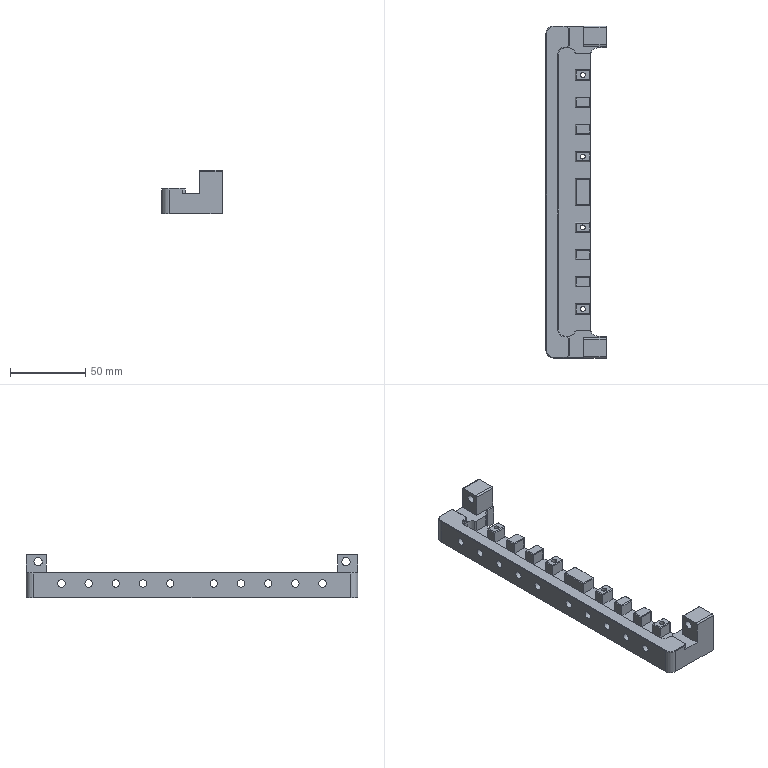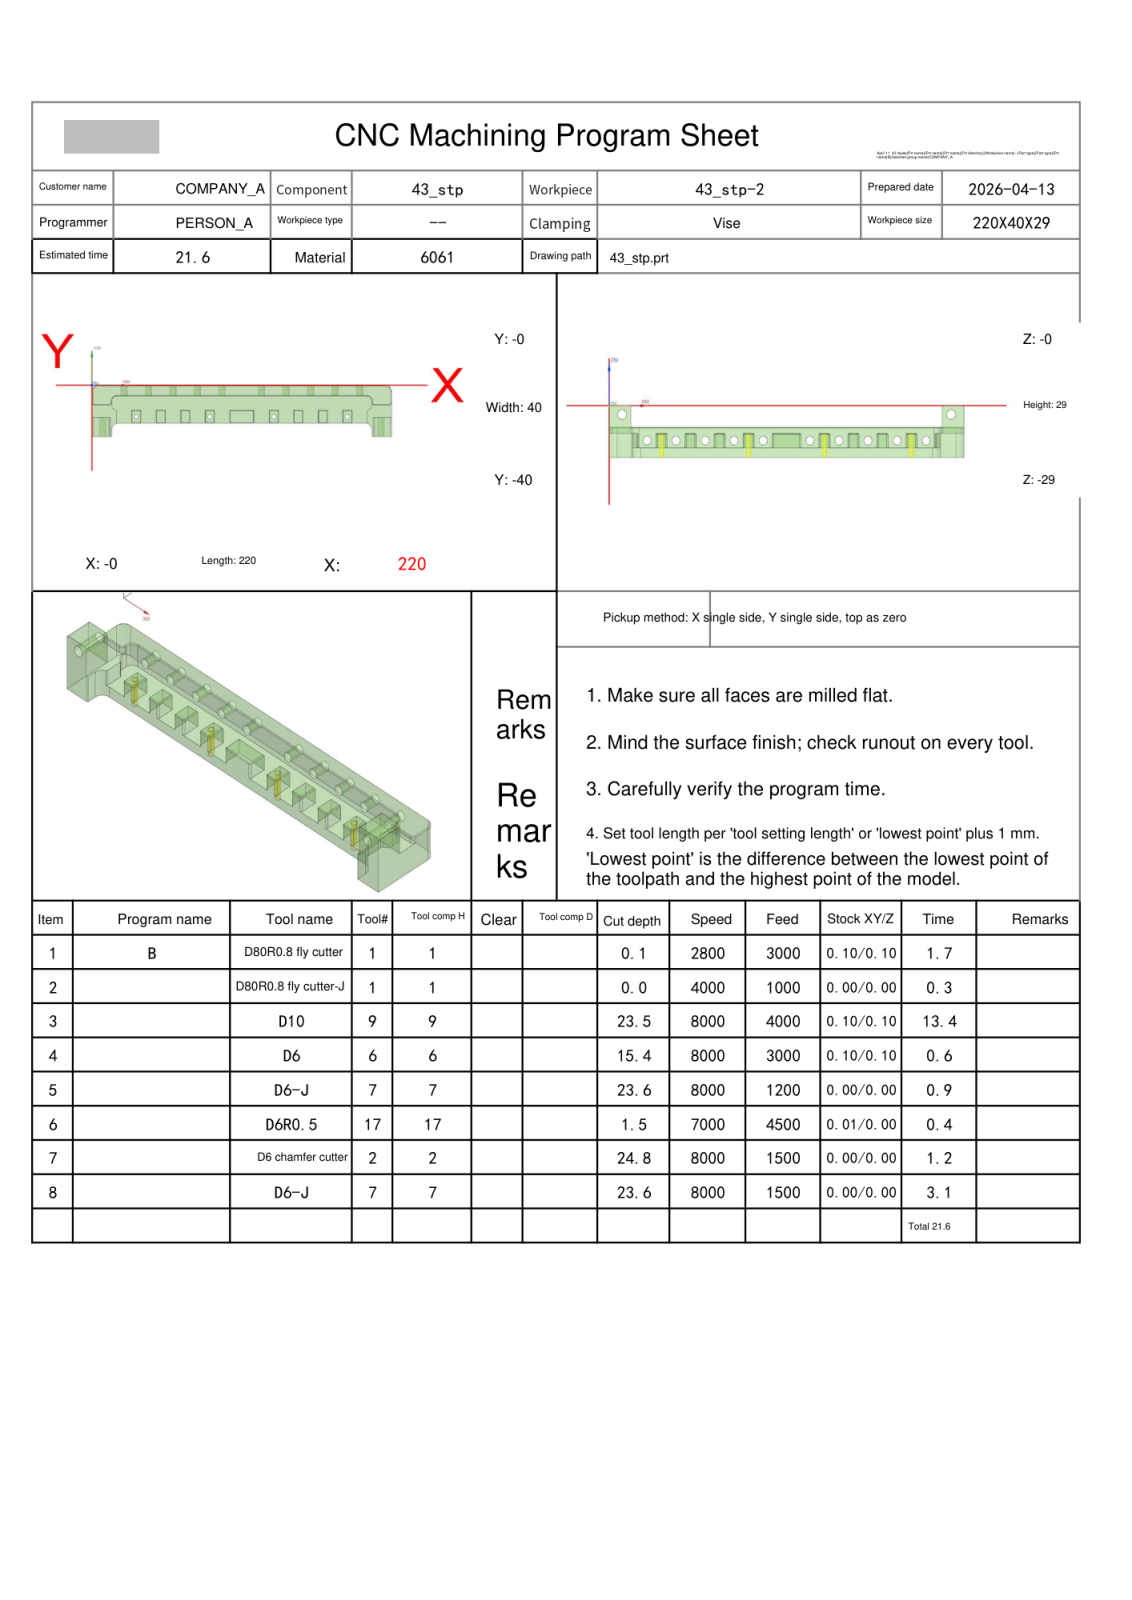NC program | NX | posted by the shop | part box 40 x 220 x 29 mm
Lines 8119 to 8430 of 14837:
N4 T06 M06
(D6  D=6. R=0. H=06 ce=0.10 di=0.10)
G00 G90 G54 X23.95 Y-27.326 M03 S8000
G43 H06 Z15.8
M08
Z-10.986
G01 Z-12.486 F3000.
X20.89
Y-29.347
X20.73 Y-30.184
X17.067 Y-41.091
X16.6 Y-41.558
Y-21.9
X-2.94
Y-14.767
G03 X2. Y-18.6 I4.94 J1.267
G01 X12.5
G03 X17.6 Y-13.5 I0.0 J5.1
G01 Y-13.074
X20.732 Y-19.026
X20.89 Y-20.022
Y-27.326
Y-27.826
X23.95
Z-10.986
G00 Y-27.326
Z-11.471
G01 Z-12.971
X20.89
Y-29.347
X20.73 Y-30.184
X17.067 Y-41.091
X16.6 Y-41.558
Y-21.9
X-2.94
Y-14.767
G03 X2. Y-18.6 I4.94 J1.267
G01 X12.5
G03 X17.6 Y-13.5 I0.0 J5.1
G01 Y-13.074
X20.732 Y-19.026
X20.89 Y-20.022
Y-27.326
Y-27.826
X23.95
Z-11.471
G00 Y-27.326
Z-11.957
G01 Z-13.457
X20.89
Y-29.347
X20.73 Y-30.184
X17.067 Y-41.091
X16.6 Y-41.558
Y-21.9
X-2.94
Y-14.767
G03 X2. Y-18.6 I4.94 J1.267
G01 X12.5
G03 X17.6 Y-13.5 I0.0 J5.1
G01 Y-13.074
X20.732 Y-19.026
X20.89 Y-20.022
Y-27.326
Y-27.826
X23.95
Z-11.957
G00 Y-27.326
Z-12.443
G01 Z-13.943
X20.89
Y-29.347
X20.73 Y-30.184
X17.067 Y-41.091
X16.6 Y-41.558
Y-21.9
X-2.94
Y-14.767
G03 X2. Y-18.6 I4.94 J1.267
G01 X12.5
G03 X17.6 Y-13.5 I0.0 J5.1
G01 Y-13.074
X20.732 Y-19.026
X20.89 Y-20.022
Y-27.326
Y-27.826
X23.95
Z-12.443
G00 Y-27.326
Z-12.929
G01 Z-14.429
X20.89
Y-29.347
X20.73 Y-30.184
X17.067 Y-41.091
X16.6 Y-41.558
Y-21.9
X-2.94
Y-14.767
G03 X2. Y-18.6 I4.94 J1.267
G01 X12.5
G03 X17.6 Y-13.5 I0.0 J5.1
G01 Y-13.074
X20.732 Y-19.026
X20.89 Y-20.022
Y-27.326
Y-27.826
X23.95
Z-12.929
G00 Y-27.326
Z-13.414
G01 Z-14.914
X20.89
Y-29.347
X20.73 Y-30.184
X17.067 Y-41.091
X16.6 Y-41.558
Y-21.9
X-2.94
Y-14.767
G03 X2. Y-18.6 I4.94 J1.267
G01 X12.5
G03 X17.6 Y-13.5 I0.0 J5.1
G01 Y-13.074
X20.732 Y-19.026
X20.89 Y-20.022
Y-27.326
Y-27.826
X23.95
Z-13.414
G00 Y-27.326
Z-13.9
G01 Z-15.4
X20.89
Y-29.347
X20.73 Y-30.184
X17.067 Y-41.091
X16.6 Y-41.558
Y-21.9
X-2.94
Y-14.767
G03 X2. Y-18.6 I4.94 J1.267
G01 X12.5
G03 X17.6 Y-13.5 I0.0 J5.1
G01 Y-13.074
X20.732 Y-19.026
X20.89 Y-20.022
Y-27.326
Y-27.826
X23.95
Z-13.9
G00 Z-9.
X196.05 Y-27.94
Z-10.986
G01 Z-12.486
X199.11
Y-20.022
X199.268 Y-19.026
X199.631 Y-18.312
X202.4 Y-13.074
Y-13.5
G03 X207.5 Y-18.6 I5.1 J0.0
G01 X218.
G03 X222.94 Y-14.767 I0.0 J5.1
G01 Y-21.9
X203.4
Y-42.94
X203.354
X199.266 Y-30.164
X199.11 Y-29.347
Y-27.94
Y-27.44
X196.05
Z-10.986
G00 Y-27.94
Z-11.471
G01 Z-12.971
X199.11
Y-20.022
X199.268 Y-19.026
X199.631 Y-18.312
X202.4 Y-13.074
Y-13.5
G03 X207.5 Y-18.6 I5.1 J0.0
G01 X218.
G03 X222.94 Y-14.767 I0.0 J5.1
G01 Y-21.9
X203.4
Y-42.94
X203.354
X199.266 Y-30.164
X199.11 Y-29.347
Y-27.94
Y-27.44
X196.05
Z-11.471
G00 Y-27.94
Z-11.957
G01 Z-13.457
X199.11
Y-20.022
X199.268 Y-19.026
X199.631 Y-18.312
X202.4 Y-13.074
Y-13.5
G03 X207.5 Y-18.6 I5.1 J0.0
G01 X218.
G03 X222.94 Y-14.767 I0.0 J5.1
G01 Y-21.9
X203.4
Y-42.94
X203.354
X199.266 Y-30.164
X199.11 Y-29.347
Y-27.94
Y-27.44
X196.05
Z-11.957
G00 Y-27.94
Z-12.443
G01 Z-13.943
X199.11
Y-20.022
X199.268 Y-19.026
X199.631 Y-18.312
X202.4 Y-13.074
Y-13.5
G03 X207.5 Y-18.6 I5.1 J0.0
G01 X218.
G03 X222.94 Y-14.767 I0.0 J5.1
G01 Y-21.9
X203.4
Y-42.94
X203.354
X199.266 Y-30.164
X199.11 Y-29.347
Y-27.94
Y-27.44
X196.05
Z-12.443
G00 Y-27.94
Z-12.929
G01 Z-14.429
X199.11
Y-20.022
X199.268 Y-19.026
X199.631 Y-18.312
X202.4 Y-13.074
Y-13.5
G03 X207.5 Y-18.6 I5.1 J0.0
G01 X218.
G03 X222.94 Y-14.767 I0.0 J5.1
G01 Y-21.9
X203.4
Y-42.94
X203.354
X199.266 Y-30.164
X199.11 Y-29.347
Y-27.94
Y-27.44
X196.05
Z-12.929
G00 Y-27.94
Z-13.414
G01 Z-14.914
X199.11
Y-20.022
X199.268 Y-19.026
X199.631 Y-18.312
X202.4 Y-13.074
Y-13.5
G03 X207.5 Y-18.6 I5.1 J0.0
G01 X218.
G03 X222.94 Y-14.767 I0.0 J5.1
G01 Y-21.9
X203.4
Y-42.94
X203.354
X199.266 Y-30.164
X199.11 Y-29.347
Y-27.94
Y-27.44
X196.05
Z-13.414
G00 Y-27.94
Z-13.9
G01 Z-15.4
X199.11
Y-20.022
X199.268 Y-19.026
X199.631 Y-18.312
X202.4 Y-13.074
Y-13.5
G03 X207.5 Y-18.6 I5.1 J0.0
G01 X218.
G03 X222.94 Y-14.767 I0.0 J5.1
G01 Y-21.9
X203.4
Y-42.94
X203.354
X199.266 Y-30.164
X199.11 Y-29.347
Y-27.94
Y-27.44
X196.05
Z-13.9
G00 Z15.8
G91 G28 Z0.0
M05
M09
G91 G28 Z0.0
M01